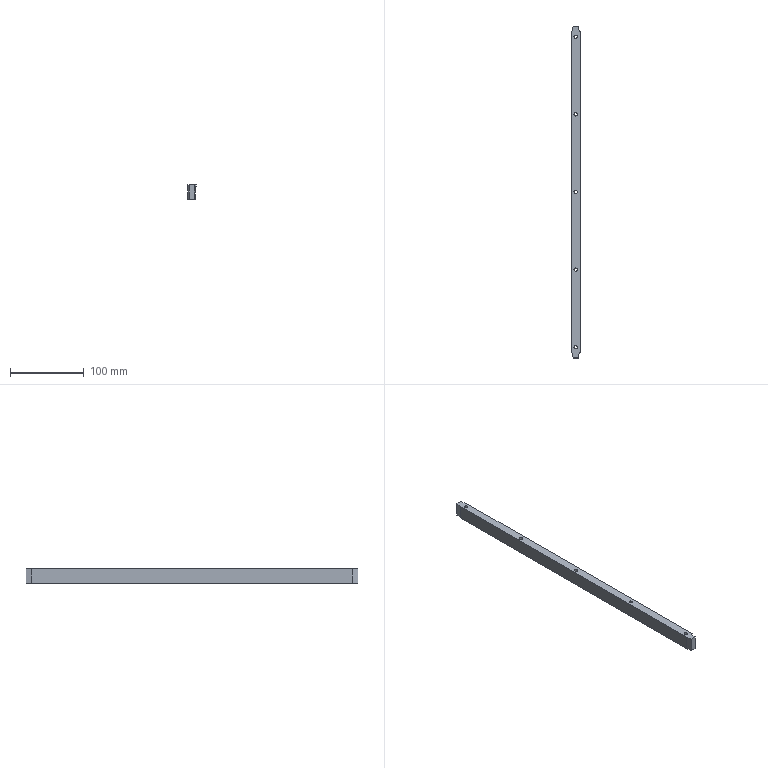Part | STEP file | 11-FG-SZ00211 | 1 solid | 39 faces | box 11 x 449 x 19 mm | volume 83756 mm3 | cylinder 20 | plane 19 | commonest cylinder face diameters 4.5 x10 8 x10
STEP:
#1=CARTESIAN_POINT('',(4.,0.,4.4));
#2=VERTEX_POINT('',#1);
#3=CARTESIAN_POINT('',(-4.,0.,4.4));
#4=VERTEX_POINT('',#3);
#5=CARTESIAN_POINT('',(0.,0.,4.4));
#6=DIRECTION('',(0.,0.,-1.));
#7=DIRECTION('',(-1.,0.,0.));
#8=AXIS2_PLACEMENT_3D('',#5,#6,#7);
#9=CIRCLE('',#8,4.);
#10=EDGE_CURVE('',#2,#4,#9,.T.);
#11=ORIENTED_EDGE('',*,*,#10,.F.);
#12=CARTESIAN_POINT('',(4.,0.,0.));
#13=VERTEX_POINT('',#12);
#14=CARTESIAN_POINT('',(4.,0.,0.));
#15=DIRECTION('',(0.,0.,-1.));
#16=VECTOR('',#15,1000.);
#17=LINE('',#14,#16);
#18=EDGE_CURVE('',#2,#13,#17,.T.);
#19=ORIENTED_EDGE('',*,*,#18,.T.);
#20=CARTESIAN_POINT('',(-4.,0.,0.));
#21=VERTEX_POINT('',#20);
#22=CARTESIAN_POINT('',(0.,0.,0.));
#23=DIRECTION('',(0.,0.,-1.));
#24=DIRECTION('',(-1.,0.,0.));
#25=AXIS2_PLACEMENT_3D('',#22,#23,#24);
#26=CIRCLE('',#25,4.);
#27=EDGE_CURVE('',#13,#21,#26,.T.);
#28=ORIENTED_EDGE('',*,*,#27,.T.);
#29=CARTESIAN_POINT('',(-4.,0.,0.));
#30=DIRECTION('',(0.,0.,-1.));
#31=VECTOR('',#30,1000.);
#32=LINE('',#29,#31);
#33=EDGE_CURVE('',#4,#21,#32,.T.);
#34=ORIENTED_EDGE('',*,*,#33,.F.);
#35=EDGE_LOOP('',(#11,#19,#28,#34));
#36=FACE_OUTER_BOUND('',#35,.T.);
#37=CARTESIAN_POINT('',(0.,0.,0.));
#38=DIRECTION('',(0.,0.,-1.));
#39=DIRECTION('',(-1.,0.,0.));
#40=AXIS2_PLACEMENT_3D('',#37,#38,#39);
#41=CYLINDRICAL_SURFACE('',#40,4.);
#42=ADVANCED_FACE('',(#36),#41,.F.);
#43=CARTESIAN_POINT('',(2.25,0.,19.));
#44=VERTEX_POINT('',#43);
#45=CARTESIAN_POINT('',(-2.25,0.,19.));
#46=VERTEX_POINT('',#45);
#47=CARTESIAN_POINT('',(0.,0.,19.));
#48=DIRECTION('',(0.,0.,-1.));
#49=DIRECTION('',(-1.,0.,0.));
#50=AXIS2_PLACEMENT_3D('',#47,#48,#49);
#51=CIRCLE('',#50,2.25);
#52=EDGE_CURVE('',#44,#46,#51,.T.);
#53=ORIENTED_EDGE('',*,*,#52,.F.);
#54=CARTESIAN_POINT('',(2.25,0.,4.4));
#55=VERTEX_POINT('',#54);
#56=CARTESIAN_POINT('',(2.25,0.,0.));
#57=DIRECTION('',(0.,0.,-1.));
#58=VECTOR('',#57,1000.);
#59=LINE('',#56,#58);
#60=EDGE_CURVE('',#44,#55,#59,.T.);
#61=ORIENTED_EDGE('',*,*,#60,.T.);
#62=CARTESIAN_POINT('',(-2.25,0.,4.4));
#63=VERTEX_POINT('',#62);
#64=CARTESIAN_POINT('',(0.,0.,4.4));
#65=DIRECTION('',(0.,0.,-1.));
#66=DIRECTION('',(-1.,0.,0.));
#67=AXIS2_PLACEMENT_3D('',#64,#65,#66);
#68=CIRCLE('',#67,2.25);
#69=EDGE_CURVE('',#55,#63,#68,.T.);
#70=ORIENTED_EDGE('',*,*,#69,.T.);
#71=CARTESIAN_POINT('',(-2.25,0.,0.));
#72=DIRECTION('',(0.,0.,-1.));
#73=VECTOR('',#72,1000.);
#74=LINE('',#71,#73);
#75=EDGE_CURVE('',#46,#63,#74,.T.);
#76=ORIENTED_EDGE('',*,*,#75,.F.);
#77=EDGE_LOOP('',(#53,#61,#70,#76));
#78=FACE_OUTER_BOUND('',#77,.T.);
#79=CARTESIAN_POINT('',(0.,0.,0.));
#80=DIRECTION('',(0.,0.,-1.));
#81=DIRECTION('',(-1.,0.,0.));
#82=AXIS2_PLACEMENT_3D('',#79,#80,#81);
#83=CYLINDRICAL_SURFACE('',#82,2.25);
#84=ADVANCED_FACE('',(#78),#83,.F.);
#85=CARTESIAN_POINT('',(4.,-105.,4.4));
#86=VERTEX_POINT('',#85);
#87=CARTESIAN_POINT('',(-4.,-105.,4.4));
#88=VERTEX_POINT('',#87);
#89=CARTESIAN_POINT('',(0.,-105.,4.4));
#90=DIRECTION('',(0.,0.,-1.));
#91=DIRECTION('',(-1.,0.,0.));
#92=AXIS2_PLACEMENT_3D('',#89,#90,#91);
#93=CIRCLE('',#92,4.);
#94=EDGE_CURVE('',#86,#88,#93,.T.);
#95=ORIENTED_EDGE('',*,*,#94,.F.);
#96=CARTESIAN_POINT('',(4.,-105.,0.));
#97=VERTEX_POINT('',#96);
#98=CARTESIAN_POINT('',(4.,-105.,0.));
#99=DIRECTION('',(0.,0.,-1.));
#100=VECTOR('',#99,1000.);
#101=LINE('',#98,#100);
#102=EDGE_CURVE('',#86,#97,#101,.T.);
#103=ORIENTED_EDGE('',*,*,#102,.T.);
#104=CARTESIAN_POINT('',(-4.,-105.,0.));
#105=VERTEX_POINT('',#104);
#106=CARTESIAN_POINT('',(0.,-105.,0.));
#107=DIRECTION('',(0.,0.,-1.));
#108=DIRECTION('',(-1.,0.,0.));
#109=AXIS2_PLACEMENT_3D('',#106,#107,#108);
#110=CIRCLE('',#109,4.);
#111=EDGE_CURVE('',#97,#105,#110,.T.);
#112=ORIENTED_EDGE('',*,*,#111,.T.);
#113=CARTESIAN_POINT('',(-4.,-105.,0.));
#114=DIRECTION('',(0.,0.,-1.));
#115=VECTOR('',#114,1000.);
#116=LINE('',#113,#115);
#117=EDGE_CURVE('',#88,#105,#116,.T.);
#118=ORIENTED_EDGE('',*,*,#117,.F.);
#119=EDGE_LOOP('',(#95,#103,#112,#118));
#120=FACE_OUTER_BOUND('',#119,.T.);
#121=CARTESIAN_POINT('',(0.,-105.,0.));
#122=DIRECTION('',(0.,0.,-1.));
#123=DIRECTION('',(-1.,0.,0.));
#124=AXIS2_PLACEMENT_3D('',#121,#122,#123);
#125=CYLINDRICAL_SURFACE('',#124,4.);
#126=ADVANCED_FACE('',(#120),#125,.F.);
#127=CARTESIAN_POINT('',(2.25,-105.,19.));
#128=VERTEX_POINT('',#127);
#129=CARTESIAN_POINT('',(-2.25,-105.,19.));
#130=VERTEX_POINT('',#129);
#131=CARTESIAN_POINT('',(0.,-105.,19.));
#132=DIRECTION('',(0.,0.,-1.));
#133=DIRECTION('',(-1.,0.,0.));
#134=AXIS2_PLACEMENT_3D('',#131,#132,#133);
#135=CIRCLE('',#134,2.25);
#136=EDGE_CURVE('',#128,#130,#135,.T.);
#137=ORIENTED_EDGE('',*,*,#136,.F.);
#138=CARTESIAN_POINT('',(2.25,-105.,4.4));
#139=VERTEX_POINT('',#138);
#140=CARTESIAN_POINT('',(2.25,-105.,0.));
#141=DIRECTION('',(0.,0.,-1.));
#142=VECTOR('',#141,1000.);
#143=LINE('',#140,#142);
#144=EDGE_CURVE('',#128,#139,#143,.T.);
#145=ORIENTED_EDGE('',*,*,#144,.T.);
#146=CARTESIAN_POINT('',(-2.25,-105.,4.4));
#147=VERTEX_POINT('',#146);
#148=CARTESIAN_POINT('',(0.,-105.,4.4));
#149=DIRECTION('',(0.,0.,-1.));
#150=DIRECTION('',(-1.,0.,0.));
#151=AXIS2_PLACEMENT_3D('',#148,#149,#150);
#152=CIRCLE('',#151,2.25);
#153=EDGE_CURVE('',#139,#147,#152,.T.);
#154=ORIENTED_EDGE('',*,*,#153,.T.);
#155=CARTESIAN_POINT('',(-2.25,-105.,0.));
#156=DIRECTION('',(0.,0.,-1.));
#157=VECTOR('',#156,1000.);
#158=LINE('',#155,#157);
#159=EDGE_CURVE('',#130,#147,#158,.T.);
#160=ORIENTED_EDGE('',*,*,#159,.F.);
#161=EDGE_LOOP('',(#137,#145,#154,#160));
#162=FACE_OUTER_BOUND('',#161,.T.);
#163=CARTESIAN_POINT('',(0.,-105.,0.));
#164=DIRECTION('',(0.,0.,-1.));
#165=DIRECTION('',(-1.,0.,0.));
#166=AXIS2_PLACEMENT_3D('',#163,#164,#165);
#167=CYLINDRICAL_SURFACE('',#166,2.25);
#168=ADVANCED_FACE('',(#162),#167,.F.);
#169=CARTESIAN_POINT('',(4.,105.,4.4));
#170=VERTEX_POINT('',#169);
#171=CARTESIAN_POINT('',(-4.,105.,4.4));
#172=VERTEX_POINT('',#171);
#173=CARTESIAN_POINT('',(0.,105.,4.4));
#174=DIRECTION('',(0.,0.,-1.));
#175=DIRECTION('',(-1.,0.,0.));
#176=AXIS2_PLACEMENT_3D('',#173,#174,#175);
#177=CIRCLE('',#176,4.);
#178=EDGE_CURVE('',#170,#172,#177,.T.);
#179=ORIENTED_EDGE('',*,*,#178,.F.);
#180=CARTESIAN_POINT('',(4.,105.,0.));
#181=VERTEX_POINT('',#180);
#182=CARTESIAN_POINT('',(4.,105.,0.));
#183=DIRECTION('',(0.,0.,-1.));
#184=VECTOR('',#183,1000.);
#185=LINE('',#182,#184);
#186=EDGE_CURVE('',#170,#181,#185,.T.);
#187=ORIENTED_EDGE('',*,*,#186,.T.);
#188=CARTESIAN_POINT('',(-4.,105.,0.));
#189=VERTEX_POINT('',#188);
#190=CARTESIAN_POINT('',(0.,105.,0.));
#191=DIRECTION('',(0.,0.,-1.));
#192=DIRECTION('',(-1.,0.,0.));
#193=AXIS2_PLACEMENT_3D('',#190,#191,#192);
#194=CIRCLE('',#193,4.);
#195=EDGE_CURVE('',#181,#189,#194,.T.);
#196=ORIENTED_EDGE('',*,*,#195,.T.);
#197=CARTESIAN_POINT('',(-4.,105.,0.));
#198=DIRECTION('',(0.,0.,-1.));
#199=VECTOR('',#198,1000.);
#200=LINE('',#197,#199);
#201=EDGE_CURVE('',#172,#189,#200,.T.);
#202=ORIENTED_EDGE('',*,*,#201,.F.);
#203=EDGE_LOOP('',(#179,#187,#196,#202));
#204=FACE_OUTER_BOUND('',#203,.T.);
#205=CARTESIAN_POINT('',(0.,105.,0.));
#206=DIRECTION('',(0.,0.,-1.));
#207=DIRECTION('',(-1.,0.,0.));
#208=AXIS2_PLACEMENT_3D('',#205,#206,#207);
#209=CYLINDRICAL_SURFACE('',#208,4.);
#210=ADVANCED_FACE('',(#204),#209,.F.);
#211=CARTESIAN_POINT('',(2.25,105.,19.));
#212=VERTEX_POINT('',#211);
#213=CARTESIAN_POINT('',(-2.25,105.,19.));
#214=VERTEX_POINT('',#213);
#215=CARTESIAN_POINT('',(0.,105.,19.));
#216=DIRECTION('',(0.,0.,-1.));
#217=DIRECTION('',(-1.,0.,0.));
#218=AXIS2_PLACEMENT_3D('',#215,#216,#217);
#219=CIRCLE('',#218,2.25);
#220=EDGE_CURVE('',#212,#214,#219,.T.);
#221=ORIENTED_EDGE('',*,*,#220,.F.);
#222=CARTESIAN_POINT('',(2.25,105.,4.4));
#223=VERTEX_POINT('',#222);
#224=CARTESIAN_POINT('',(2.25,105.,0.));
#225=DIRECTION('',(0.,0.,-1.));
#226=VECTOR('',#225,1000.);
#227=LINE('',#224,#226);
#228=EDGE_CURVE('',#212,#223,#227,.T.);
#229=ORIENTED_EDGE('',*,*,#228,.T.);
#230=CARTESIAN_POINT('',(-2.25,105.,4.4));
#231=VERTEX_POINT('',#230);
#232=CARTESIAN_POINT('',(0.,105.,4.4));
#233=DIRECTION('',(0.,0.,-1.));
#234=DIRECTION('',(-1.,0.,0.));
#235=AXIS2_PLACEMENT_3D('',#232,#233,#234);
#236=CIRCLE('',#235,2.25);
#237=EDGE_CURVE('',#223,#231,#236,.T.);
#238=ORIENTED_EDGE('',*,*,#237,.T.);
#239=CARTESIAN_POINT('',(-2.25,105.,0.));
#240=DIRECTION('',(0.,0.,-1.));
#241=VECTOR('',#240,1000.);
#242=LINE('',#239,#241);
#243=EDGE_CURVE('',#214,#231,#242,.T.);
#244=ORIENTED_EDGE('',*,*,#243,.F.);
#245=EDGE_LOOP('',(#221,#229,#238,#244));
#246=FACE_OUTER_BOUND('',#245,.T.);
#247=CARTESIAN_POINT('',(0.,105.,0.));
#248=DIRECTION('',(0.,0.,-1.));
#249=DIRECTION('',(-1.,0.,0.));
#250=AXIS2_PLACEMENT_3D('',#247,#248,#249);
#251=CYLINDRICAL_SURFACE('',#250,2.25);
#252=ADVANCED_FACE('',(#246),#251,.F.);
#253=CARTESIAN_POINT('',(4.,-210.,4.4));
#254=VERTEX_POINT('',#253);
#255=CARTESIAN_POINT('',(-4.,-210.,4.4));
#256=VERTEX_POINT('',#255);
#257=CARTESIAN_POINT('',(0.,-210.,4.4));
#258=DIRECTION('',(0.,0.,-1.));
#259=DIRECTION('',(-1.,0.,0.));
#260=AXIS2_PLACEMENT_3D('',#257,#258,#259);
#261=CIRCLE('',#260,4.);
#262=EDGE_CURVE('',#254,#256,#261,.T.);
#263=ORIENTED_EDGE('',*,*,#262,.F.);
#264=CARTESIAN_POINT('',(4.,-210.,0.));
#265=VERTEX_POINT('',#264);
#266=CARTESIAN_POINT('',(4.,-210.,0.));
#267=DIRECTION('',(0.,0.,-1.));
#268=VECTOR('',#267,1000.);
#269=LINE('',#266,#268);
#270=EDGE_CURVE('',#254,#265,#269,.T.);
#271=ORIENTED_EDGE('',*,*,#270,.T.);
#272=CARTESIAN_POINT('',(-4.,-210.,0.));
#273=VERTEX_POINT('',#272);
#274=CARTESIAN_POINT('',(0.,-210.,0.));
#275=DIRECTION('',(0.,0.,-1.));
#276=DIRECTION('',(-1.,0.,0.));
#277=AXIS2_PLACEMENT_3D('',#274,#275,#276);
#278=CIRCLE('',#277,4.);
#279=EDGE_CURVE('',#265,#273,#278,.T.);
#280=ORIENTED_EDGE('',*,*,#279,.T.);
#281=CARTESIAN_POINT('',(-4.,-210.,0.));
#282=DIRECTION('',(0.,0.,-1.));
#283=VECTOR('',#282,1000.);
#284=LINE('',#281,#283);
#285=EDGE_CURVE('',#256,#273,#284,.T.);
#286=ORIENTED_EDGE('',*,*,#285,.F.);
#287=EDGE_LOOP('',(#263,#271,#280,#286));
#288=FACE_OUTER_BOUND('',#287,.T.);
#289=CARTESIAN_POINT('',(0.,-210.,0.));
#290=DIRECTION('',(0.,0.,-1.));
#291=DIRECTION('',(-1.,0.,0.));
#292=AXIS2_PLACEMENT_3D('',#289,#290,#291);
#293=CYLINDRICAL_SURFACE('',#292,4.);
#294=ADVANCED_FACE('',(#288),#293,.F.);
#295=CARTESIAN_POINT('',(2.25,-210.,19.));
#296=VERTEX_POINT('',#295);
#297=CARTESIAN_POINT('',(-2.25,-210.,19.));
#298=VERTEX_POINT('',#297);
#299=CARTESIAN_POINT('',(0.,-210.,19.));
#300=DIRECTION('',(0.,0.,-1.));
#301=DIRECTION('',(-1.,0.,0.));
#302=AXIS2_PLACEMENT_3D('',#299,#300,#301);
#303=CIRCLE('',#302,2.25);
#304=EDGE_CURVE('',#296,#298,#303,.T.);
#305=ORIENTED_EDGE('',*,*,#304,.F.);
#306=CARTESIAN_POINT('',(2.25,-210.,4.4));
#307=VERTEX_POINT('',#306);
#308=CARTESIAN_POINT('',(2.25,-210.,0.));
#309=DIRECTION('',(0.,0.,-1.));
#310=VECTOR('',#309,1000.);
#311=LINE('',#308,#310);
#312=EDGE_CURVE('',#296,#307,#311,.T.);
#313=ORIENTED_EDGE('',*,*,#312,.T.);
#314=CARTESIAN_POINT('',(-2.25,-210.,4.4));
#315=VERTEX_POINT('',#314);
#316=CARTESIAN_POINT('',(0.,-210.,4.4));
#317=DIRECTION('',(0.,0.,-1.));
#318=DIRECTION('',(-1.,0.,0.));
#319=AXIS2_PLACEMENT_3D('',#316,#317,#318);
#320=CIRCLE('',#319,2.25);
#321=EDGE_CURVE('',#307,#315,#320,.T.);
#322=ORIENTED_EDGE('',*,*,#321,.T.);
#323=CARTESIAN_POINT('',(-2.25,-210.,0.));
#324=DIRECTION('',(0.,0.,-1.));
#325=VECTOR('',#324,1000.);
#326=LINE('',#323,#325);
#327=EDGE_CURVE('',#298,#315,#326,.T.);
#328=ORIENTED_EDGE('',*,*,#327,.F.);
#329=EDGE_LOOP('',(#305,#313,#322,#328));
#330=FACE_OUTER_BOUND('',#329,.T.);
#331=CARTESIAN_POINT('',(0.,-210.,0.));
#332=DIRECTION('',(0.,0.,-1.));
#333=DIRECTION('',(-1.,0.,0.));
#334=AXIS2_PLACEMENT_3D('',#331,#332,#333);
#335=CYLINDRICAL_SURFACE('',#334,2.25);
#336=ADVANCED_FACE('',(#330),#335,.F.);
#337=CARTESIAN_POINT('',(4.,210.,4.4));
#338=VERTEX_POINT('',#337);
#339=CARTESIAN_POINT('',(-4.,210.,4.4));
#340=VERTEX_POINT('',#339);
#341=CARTESIAN_POINT('',(0.,210.,4.4));
#342=DIRECTION('',(0.,0.,-1.));
#343=DIRECTION('',(-1.,0.,0.));
#344=AXIS2_PLACEMENT_3D('',#341,#342,#343);
#345=CIRCLE('',#344,4.);
#346=EDGE_CURVE('',#338,#340,#345,.T.);
#347=ORIENTED_EDGE('',*,*,#346,.F.);
#348=CARTESIAN_POINT('',(4.,210.,0.));
#349=VERTEX_POINT('',#348);
#350=CARTESIAN_POINT('',(4.,210.,0.));
#351=DIRECTION('',(0.,0.,-1.));
#352=VECTOR('',#351,1000.);
#353=LINE('',#350,#352);
#354=EDGE_CURVE('',#338,#349,#353,.T.);
#355=ORIENTED_EDGE('',*,*,#354,.T.);
#356=CARTESIAN_POINT('',(-4.,210.,0.));
#357=VERTEX_POINT('',#356);
#358=CARTESIAN_POINT('',(0.,210.,0.));
#359=DIRECTION('',(0.,0.,-1.));
#360=DIRECTION('',(-1.,0.,0.));
#361=AXIS2_PLACEMENT_3D('',#358,#359,#360);
#362=CIRCLE('',#361,4.);
#363=EDGE_CURVE('',#349,#357,#362,.T.);
#364=ORIENTED_EDGE('',*,*,#363,.T.);
#365=CARTESIAN_POINT('',(-4.,210.,0.));
#366=DIRECTION('',(0.,0.,-1.));
#367=VECTOR('',#366,1000.);
#368=LINE('',#365,#367);
#369=EDGE_CURVE('',#340,#357,#368,.T.);
#370=ORIENTED_EDGE('',*,*,#369,.F.);
#371=EDGE_LOOP('',(#347,#355,#364,#370));
#372=FACE_OUTER_BOUND('',#371,.T.);
#373=CARTESIAN_POINT('',(0.,210.,0.));
#374=DIRECTION('',(0.,0.,-1.));
#375=DIRECTION('',(-1.,0.,0.));
#376=AXIS2_PLACEMENT_3D('',#373,#374,#375);
#377=CYLINDRICAL_SURFACE('',#376,4.);
#378=ADVANCED_FACE('',(#372),#377,.F.);
#379=CARTESIAN_POINT('',(2.25,210.,19.));
#380=VERTEX_POINT('',#379);
#381=CARTESIAN_POINT('',(-2.25,210.,19.));
#382=VERTEX_POINT('',#381);
#383=CARTESIAN_POINT('',(0.,210.,19.));
#384=DIRECTION('',(0.,0.,-1.));
#385=DIRECTION('',(-1.,0.,0.));
#386=AXIS2_PLACEMENT_3D('',#383,#384,#385);
#387=CIRCLE('',#386,2.25);
#388=EDGE_CURVE('',#380,#382,#387,.T.);
#389=ORIENTED_EDGE('',*,*,#388,.F.);
#390=CARTESIAN_POINT('',(2.25,210.,4.4));
#391=VERTEX_POINT('',#390);
#392=CARTESIAN_POINT('',(2.25,210.,0.));
#393=DIRECTION('',(0.,0.,-1.));
#394=VECTOR('',#393,1000.);
#395=LINE('',#392,#394);
#396=EDGE_CURVE('',#380,#391,#395,.T.);
#397=ORIENTED_EDGE('',*,*,#396,.T.);
#398=CARTESIAN_POINT('',(-2.25,210.,4.4));
#399=VERTEX_POINT('',#398);
#400=CARTESIAN_POINT('',(0.,210.,4.4));
#401=DIRECTION('',(0.,0.,-1.));
#402=DIRECTION('',(-1.,0.,0.));
#403=AXIS2_PLACEMENT_3D('',#400,#401,#402);
#404=CIRCLE('',#403,2.25);
#405=EDGE_CURVE('',#391,#399,#404,.T.);
#406=ORIENTED_EDGE('',*,*,#405,.T.);
#407=CARTESIAN_POINT('',(-2.25,210.,0.));
#408=DIRECTION('',(0.,0.,-1.));
#409=VECTOR('',#408,1000.);
#410=LINE('',#407,#409);
#411=EDGE_CURVE('',#382,#399,#410,.T.);
#412=ORIENTED_EDGE('',*,*,#411,.F.);
#413=EDGE_LOOP('',(#389,#397,#406,#412));
#414=FACE_OUTER_BOUND('',#413,.T.);
#415=CARTESIAN_POINT('',(0.,210.,0.));
#416=DIRECTION('',(0.,0.,-1.));
#417=DIRECTION('',(-1.,0.,0.));
#418=AXIS2_PLACEMENT_3D('',#415,#416,#417);
#419=CYLINDRICAL_SURFACE('',#418,2.25);
#420=ADVANCED_FACE('',(#414),#419,.F.);
#421=CARTESIAN_POINT('',(5.,-216.5,16.3));
#422=VERTEX_POINT('',#421);
#423=CARTESIAN_POINT('',(5.,216.5,16.3));
#424=VERTEX_POINT('',#423);
#425=CARTESIAN_POINT('',(5.,-216.5,16.3));
#426=DIRECTION('',(0.,1.,0.));
#427=VECTOR('',#426,1000.);
#428=LINE('',#425,#427);
#429=EDGE_CURVE('',#422,#424,#428,.T.);
#430=ORIENTED_EDGE('',*,*,#429,.F.);
#431=CARTESIAN_POINT('',(5.,-216.5,0.));
#432=VERTEX_POINT('',#431);
#433=CARTESIAN_POINT('',(5.,-216.5,19.));
#434=DIRECTION('',(0.,0.,-1.));
#435=VECTOR('',#434,1000.);
#436=LINE('',#433,#435);
#437=EDGE_CURVE('',#422,#432,#436,.T.);
#438=ORIENTED_EDGE('',*,*,#437,.T.);
#439=CARTESIAN_POINT('',(5.,216.5,0.));
#440=VERTEX_POINT('',#439);
#441=CARTESIAN_POINT('',(5.,224.5,0.));
#442=DIRECTION('',(0.,1.,0.));
#443=VECTOR('',#442,1000.);
#444=LINE('',#441,#443);
#445=EDGE_CURVE('',#432,#440,#444,.T.);
#446=ORIENTED_EDGE('',*,*,#445,.T.);
#447=CARTESIAN_POINT('',(5.,216.5,19.));
#448=DIRECTION('',(0.,0.,1.));
#449=VECTOR('',#448,1000.);
#450=LINE('',#447,#449);
#451=EDGE_CURVE('',#440,#424,#450,.T.);
#452=ORIENTED_EDGE('',*,*,#451,.T.);
#453=EDGE_LOOP('',(#430,#438,#446,#452));
#454=FACE_OUTER_BOUND('',#453,.T.);
#455=CARTESIAN_POINT('',(5.,224.5,19.));
#456=DIRECTION('',(-1.,0.,0.));
#457=DIRECTION('',(0.,-1.,0.));
#458=AXIS2_PLACEMENT_3D('',#455,#456,#457);
#459=PLANE('',#458);
#460=ADVANCED_FACE('',(#454),#459,.F.);
#461=CARTESIAN_POINT('',(-5.,216.5,0.));
#462=VERTEX_POINT('',#461);
#463=CARTESIAN_POINT('',(-5.,-216.5,0.));
#464=VERTEX_POINT('',#463);
#465=CARTESIAN_POINT('',(-5.,224.5,0.));
#466=DIRECTION('',(0.,-1.,0.));
#467=VECTOR('',#466,1000.);
#468=LINE('',#465,#467);
#469=EDGE_CURVE('',#462,#464,#468,.T.);
#470=ORIENTED_EDGE('',*,*,#469,.T.);
#471=CARTESIAN_POINT('',(-5.,-216.5,19.));
#472=VERTEX_POINT('',#471);
#473=CARTESIAN_POINT('',(-5.,-216.5,19.));
#474=DIRECTION('',(0.,0.,1.));
#475=VECTOR('',#474,1000.);
#476=LINE('',#473,#475);
#477=EDGE_CURVE('',#464,#472,#476,.T.);
#478=ORIENTED_EDGE('',*,*,#477,.T.);
#479=CARTESIAN_POINT('',(-5.,216.5,19.));
#480=VERTEX_POINT('',#479);
#481=CARTESIAN_POINT('',(-5.,224.5,19.));
#482=DIRECTION('',(0.,-1.,0.));
#483=VECTOR('',#482,1000.);
#484=LINE('',#481,#483);
#485=EDGE_CURVE('',#480,#472,#484,.T.);
#486=ORIENTED_EDGE('',*,*,#485,.F.);
#487=CARTESIAN_POINT('',(-5.,216.5,19.));
#488=DIRECTION('',(0.,0.,-1.));
#489=VECTOR('',#488,1000.);
#490=LINE('',#487,#489);
#491=EDGE_CURVE('',#480,#462,#490,.T.);
#492=ORIENTED_EDGE('',*,*,#491,.T.);
#493=EDGE_LOOP('',(#470,#478,#486,#492));
#494=FACE_OUTER_BOUND('',#493,.T.);
#495=CARTESIAN_POINT('',(-5.,224.5,19.));
#496=DIRECTION('',(1.,0.,0.));
#497=DIRECTION('',(0.,1.,0.));
#498=AXIS2_PLACEMENT_3D('',#495,#496,#497);
#499=PLANE('',#498);
#500=ADVANCED_FACE('',(#494),#499,.F.);
#501=CARTESIAN_POINT('',(-3.5,-224.5,19.));
#502=VERTEX_POINT('',#501);
#503=CARTESIAN_POINT('',(3.5,-224.5,19.));
#504=VERTEX_POINT('',#503);
#505=CARTESIAN_POINT('',(5.,-224.5,19.));
#506=DIRECTION('',(1.,0.,0.));
#507=VECTOR('',#506,1000.);
#508=LINE('',#505,#507);
#509=EDGE_CURVE('',#502,#504,#508,.T.);
#510=ORIENTED_EDGE('',*,*,#509,.F.);
#511=CARTESIAN_POINT('',(-3.5,-224.5,0.));
#512=VERTEX_POINT('',#511);
#513=CARTESIAN_POINT('',(-3.5,-224.5,19.));
#514=DIRECTION('',(0.,0.,-1.));
#515=VECTOR('',#514,1000.);
#516=LINE('',#513,#515);
#517=EDGE_CURVE('',#502,#512,#516,.T.);
#518=ORIENTED_EDGE('',*,*,#517,.T.);
#519=CARTESIAN_POINT('',(3.5,-224.5,0.));
#520=VERTEX_POINT('',#519);
#521=CARTESIAN_POINT('',(5.,-224.5,0.));
#522=DIRECTION('',(1.,0.,0.));
#523=VECTOR('',#522,1000.);
#524=LINE('',#521,#523);
#525=EDGE_CURVE('',#512,#520,#524,.T.);
#526=ORIENTED_EDGE('',*,*,#525,.T.);
#527=CARTESIAN_POINT('',(3.5,-224.5,19.));
#528=DIRECTION('',(0.,0.,1.));
#529=VECTOR('',#528,1000.);
#530=LINE('',#527,#529);
#531=EDGE_CURVE('',#520,#504,#530,.T.);
#532=ORIENTED_EDGE('',*,*,#531,.T.);
#533=EDGE_LOOP('',(#510,#518,#526,#532));
#534=FACE_OUTER_BOUND('',#533,.T.);
#535=CARTESIAN_POINT('',(5.,-224.5,19.));
#536=DIRECTION('',(0.,1.,0.));
#537=DIRECTION('',(0.,0.,1.));
#538=AXIS2_PLACEMENT_3D('',#535,#536,#537);
#539=PLANE('',#538);
#540=ADVANCED_FACE('',(#534),#539,.F.);
#541=CARTESIAN_POINT('',(3.5,224.5,19.));
#542=VERTEX_POINT('',#541);
#543=CARTESIAN_POINT('',(-3.5,224.5,19.));
#544=VERTEX_POINT('',#543);
#545=CARTESIAN_POINT('',(5.,224.5,19.));
#546=DIRECTION('',(-1.,0.,0.));
#547=VECTOR('',#546,1000.);
#548=LINE('',#545,#547);
#549=EDGE_CURVE('',#542,#544,#548,.T.);
#550=ORIENTED_EDGE('',*,*,#549,.F.);
#551=CARTESIAN_POINT('',(3.5,224.5,0.));
#552=VERTEX_POINT('',#551);
#553=CARTESIAN_POINT('',(3.5,224.5,19.));
#554=DIRECTION('',(0.,0.,-1.));
#555=VECTOR('',#554,1000.);
#556=LINE('',#553,#555);
#557=EDGE_CURVE('',#542,#552,#556,.T.);
#558=ORIENTED_EDGE('',*,*,#557,.T.);
#559=CARTESIAN_POINT('',(-3.5,224.5,0.));
#560=VERTEX_POINT('',#559);
#561=CARTESIAN_POINT('',(5.,224.5,0.));
#562=DIRECTION('',(-1.,0.,0.));
#563=VECTOR('',#562,1000.);
#564=LINE('',#561,#563);
#565=EDGE_CURVE('',#552,#560,#564,.T.);
#566=ORIENTED_EDGE('',*,*,#565,.T.);
#567=CARTESIAN_POINT('',(-3.5,224.5,19.));
#568=DIRECTION('',(0.,0.,1.));
#569=VECTOR('',#568,1000.);
#570=LINE('',#567,#569);
#571=EDGE_CURVE('',#560,#544,#570,.T.);
#572=ORIENTED_EDGE('',*,*,#571,.T.);
#573=EDGE_LOOP('',(#550,#558,#566,#572));
#574=FACE_OUTER_BOUND('',#573,.T.);
#575=CARTESIAN_POINT('',(5.,224.5,19.));
#576=DIRECTION('',(0.,-1.,0.));
#577=DIRECTION('',(0.,0.,-1.));
#578=AXIS2_PLACEMENT_3D('',#575,#576,#577);
#579=PLANE('',#578);
#580=ADVANCED_FACE('',(#574),#579,.F.);
#581=CARTESIAN_POINT('',(0.,0.,19.));
#582=DIRECTION('',(0.,0.,-1.));
#583=DIRECTION('',(-1.,0.,0.));
#584=AXIS2_PLACEMENT_3D('',#581,#582,#583);
#585=CIRCLE('',#584,2.25);
#586=EDGE_CURVE('',#46,#44,#585,.T.);
#587=ORIENTED_EDGE('',*,*,#586,.T.);
#588=ORIENTED_EDGE('',*,*,#52,.T.);
#589=EDGE_LOOP('',(#587,#588));
#590=FACE_BOUND('',#589,.T.);
#591=CARTESIAN_POINT('',(0.,-105.,19.));
#592=DIRECTION('',(0.,0.,-1.));
#593=DIRECTION('',(-1.,0.,0.));
#594=AXIS2_PLACEMENT_3D('',#591,#592,#593);
#595=CIRCLE('',#594,2.25);
#596=EDGE_CURVE('',#130,#128,#595,.T.);
#597=ORIENTED_EDGE('',*,*,#596,.T.);
#598=ORIENTED_EDGE('',*,*,#136,.T.);
#599=EDGE_LOOP('',(#597,#598));
#600=FACE_BOUND('',#599,.T.);
#601=CARTESIAN_POINT('',(0.,105.,19.));
#602=DIRECTION('',(0.,0.,-1.));
#603=DIRECTION('',(-1.,0.,0.));
#604=AXIS2_PLACEMENT_3D('',#601,#602,#603);
#605=CIRCLE('',#604,2.25);
#606=EDGE_CURVE('',#214,#212,#605,.T.);
#607=ORIENTED_EDGE('',*,*,#606,.T.);
#608=ORIENTED_EDGE('',*,*,#220,.T.);
#609=EDGE_LOOP('',(#607,#608));
#610=FACE_BOUND('',#609,.T.);
#611=CARTESIAN_POINT('',(0.,-210.,19.));
#612=DIRECTION('',(0.,0.,-1.));
#613=DIRECTION('',(-1.,0.,0.));
#614=AXIS2_PLACEMENT_3D('',#611,#612,#613);
#615=CIRCLE('',#614,2.25);
#616=EDGE_CURVE('',#298,#296,#615,.T.);
#617=ORIENTED_EDGE('',*,*,#616,.T.);
#618=ORIENTED_EDGE('',*,*,#304,.T.);
#619=EDGE_LOOP('',(#617,#618));
#620=FACE_BOUND('',#619,.T.);
#621=CARTESIAN_POINT('',(0.,210.,19.));
#622=DIRECTION('',(0.,0.,-1.));
#623=DIRECTION('',(-1.,0.,0.));
#624=AXIS2_PLACEMENT_3D('',#621,#622,#623);
#625=CIRCLE('',#624,2.25);
#626=EDGE_CURVE('',#382,#380,#625,.T.);
#627=ORIENTED_EDGE('',*,*,#626,.T.);
#628=ORIENTED_EDGE('',*,*,#388,.T.);
#629=EDGE_LOOP('',(#627,#628));
#630=FACE_BOUND('',#629,.T.);
#631=CARTESIAN_POINT('',(5.,-216.5,19.));
#632=VERTEX_POINT('',#631);
#633=CARTESIAN_POINT('',(5.,-216.5,19.));
#634=DIRECTION('',(0.1843,0.9829,0.));
#635=VECTOR('',#634,1000.);
#636=LINE('',#633,#635);
#637=EDGE_CURVE('',#504,#632,#636,.T.);
#638=ORIENTED_EDGE('',*,*,#637,.T.);
#639=CARTESIAN_POINT('',(6.,-216.5,19.));
#640=VERTEX_POINT('',#639);
#641=CARTESIAN_POINT('',(6.,-216.5,19.));
#642=DIRECTION('',(-1.,0.,0.));
#643=VECTOR('',#642,1000.);
#644=LINE('',#641,#643);
#645=EDGE_CURVE('',#640,#632,#644,.T.);
#646=ORIENTED_EDGE('',*,*,#645,.F.);
#647=CARTESIAN_POINT('',(6.,216.5,19.));
#648=VERTEX_POINT('',#647);
#649=CARTESIAN_POINT('',(6.,-216.5,19.));
#650=DIRECTION('',(0.,-1.,0.));
#651=VECTOR('',#650,1000.);
#652=LINE('',#649,#651);
#653=EDGE_CURVE('',#648,#640,#652,.T.);
#654=ORIENTED_EDGE('',*,*,#653,.F.);
#655=CARTESIAN_POINT('',(5.,216.5,19.));
#656=VERTEX_POINT('',#655);
#657=CARTESIAN_POINT('',(6.,216.5,19.));
#658=DIRECTION('',(-1.,0.,0.));
#659=VECTOR('',#658,1000.);
#660=LINE('',#657,#659);
#661=EDGE_CURVE('',#648,#656,#660,.T.);
#662=ORIENTED_EDGE('',*,*,#661,.T.);
#663=CARTESIAN_POINT('',(3.5,224.5,19.));
#664=DIRECTION('',(-0.1843,0.9829,0.));
#665=VECTOR('',#664,1000.);
#666=LINE('',#663,#665);
#667=EDGE_CURVE('',#656,#542,#666,.T.);
#668=ORIENTED_EDGE('',*,*,#667,.T.);
#669=ORIENTED_EDGE('',*,*,#549,.T.);
#670=CARTESIAN_POINT('',(-5.,216.5,19.));
#671=DIRECTION('',(-0.1843,-0.9829,0.));
#672=VECTOR('',#671,1000.);
#673=LINE('',#670,#672);
#674=EDGE_CURVE('',#544,#480,#673,.T.);
#675=ORIENTED_EDGE('',*,*,#674,.T.);
#676=ORIENTED_EDGE('',*,*,#485,.T.);
#677=CARTESIAN_POINT('',(-3.5,-224.5,19.));
#678=DIRECTION('',(0.1843,-0.9829,0.));
#679=VECTOR('',#678,1000.);
#680=LINE('',#677,#679);
#681=EDGE_CURVE('',#472,#502,#680,.T.);
#682=ORIENTED_EDGE('',*,*,#681,.T.);
#683=ORIENTED_EDGE('',*,*,#509,.T.);
#684=EDGE_LOOP('',(#638,#646,#654,#662,#668,#669,#675,#676,#682,#683));
#685=FACE_OUTER_BOUND('',#684,.T.);
#686=CARTESIAN_POINT('',(0.,0.,19.));
#687=DIRECTION('',(0.,0.,-1.));
#688=DIRECTION('',(-1.,0.,0.));
#689=AXIS2_PLACEMENT_3D('',#686,#687,#688);
#690=PLANE('',#689);
#691=ADVANCED_FACE('',(#590,#600,#610,#620,#630,#685),#690,.F.);
#692=CARTESIAN_POINT('',(0.,0.,0.));
#693=DIRECTION('',(0.,0.,-1.));
#694=DIRECTION('',(-1.,0.,0.));
#695=AXIS2_PLACEMENT_3D('',#692,#693,#694);
#696=CIRCLE('',#695,4.);
#697=EDGE_CURVE('',#21,#13,#696,.T.);
#698=ORIENTED_EDGE('',*,*,#697,.F.);
#699=ORIENTED_EDGE('',*,*,#27,.F.);
#700=EDGE_LOOP('',(#698,#699));
#701=FACE_BOUND('',#700,.T.);
#702=CARTESIAN_POINT('',(0.,-105.,0.));
#703=DIRECTION('',(0.,0.,-1.));
#704=DIRECTION('',(-1.,0.,0.));
#705=AXIS2_PLACEMENT_3D('',#702,#703,#704);
#706=CIRCLE('',#705,4.);
#707=EDGE_CURVE('',#105,#97,#706,.T.);
#708=ORIENTED_EDGE('',*,*,#707,.F.);
#709=ORIENTED_EDGE('',*,*,#111,.F.);
#710=EDGE_LOOP('',(#708,#709));
#711=FACE_BOUND('',#710,.T.);
#712=CARTESIAN_POINT('',(0.,105.,0.));
#713=DIRECTION('',(0.,0.,-1.));
#714=DIRECTION('',(-1.,0.,0.));
#715=AXIS2_PLACEMENT_3D('',#712,#713,#714);
#716=CIRCLE('',#715,4.);
#717=EDGE_CURVE('',#189,#181,#716,.T.);
#718=ORIENTED_EDGE('',*,*,#717,.F.);
#719=ORIENTED_EDGE('',*,*,#195,.F.);
#720=EDGE_LOOP('',(#718,#719));
#721=FACE_BOUND('',#720,.T.);
#722=CARTESIAN_POINT('',(0.,-210.,0.));
#723=DIRECTION('',(0.,0.,-1.));
#724=DIRECTION('',(-1.,0.,0.));
#725=AXIS2_PLACEMENT_3D('',#722,#723,#724);
#726=CIRCLE('',#725,4.);
#727=EDGE_CURVE('',#273,#265,#726,.T.);
#728=ORIENTED_EDGE('',*,*,#727,.F.);
#729=ORIENTED_EDGE('',*,*,#279,.F.);
#730=EDGE_LOOP('',(#728,#729));
#731=FACE_BOUND('',#730,.T.);
#732=CARTESIAN_POINT('',(0.,210.,0.));
#733=DIRECTION('',(0.,0.,-1.));
#734=DIRECTION('',(-1.,0.,0.));
#735=AXIS2_PLACEMENT_3D('',#732,#733,#734);
#736=CIRCLE('',#735,4.);
#737=EDGE_CURVE('',#357,#349,#736,.T.);
#738=ORIENTED_EDGE('',*,*,#737,.F.);
#739=ORIENTED_EDGE('',*,*,#363,.F.);
#740=EDGE_LOOP('',(#738,#739));
#741=FACE_BOUND('',#740,.T.);
#742=ORIENTED_EDGE('',*,*,#565,.F.);
#743=CARTESIAN_POINT('',(44.045,8.258,0.));
#744=DIRECTION('',(0.1843,-0.9829,0.));
#745=VECTOR('',#744,1000.);
#746=LINE('',#743,#745);
#747=EDGE_CURVE('',#552,#440,#746,.T.);
#748=ORIENTED_EDGE('',*,*,#747,.T.);
#749=ORIENTED_EDGE('',*,*,#445,.F.);
#750=CARTESIAN_POINT('',(44.045,-8.258,0.));
#751=DIRECTION('',(-0.1843,-0.9829,0.));
#752=VECTOR('',#751,1000.);
#753=LINE('',#750,#752);
#754=EDGE_CURVE('',#432,#520,#753,.T.);
#755=ORIENTED_EDGE('',*,*,#754,.T.);
#756=ORIENTED_EDGE('',*,*,#525,.F.);
#757=CARTESIAN_POINT('',(-44.045,-8.258,0.));
#758=DIRECTION('',(-0.1843,0.9829,0.));
#759=VECTOR('',#758,1000.);
#760=LINE('',#757,#759);
#761=EDGE_CURVE('',#512,#464,#760,.T.);
#762=ORIENTED_EDGE('',*,*,#761,.T.);
#763=ORIENTED_EDGE('',*,*,#469,.F.);
#764=CARTESIAN_POINT('',(-44.045,8.258,0.));
#765=DIRECTION('',(0.1843,0.9829,0.));
#766=VECTOR('',#765,1000.);
#767=LINE('',#764,#766);
#768=EDGE_CURVE('',#462,#560,#767,.T.);
#769=ORIENTED_EDGE('',*,*,#768,.T.);
#770=EDGE_LOOP('',(#742,#748,#749,#755,#756,#762,#763,#769));
#771=FACE_OUTER_BOUND('',#770,.T.);
#772=CARTESIAN_POINT('',(0.,0.,0.));
#773=DIRECTION('',(0.,0.,-1.));
#774=DIRECTION('',(-1.,0.,0.));
#775=AXIS2_PLACEMENT_3D('',#772,#773,#774);
#776=PLANE('',#775);
#777=ADVANCED_FACE('',(#701,#711,#721,#731,#741,#771),#776,.T.);
#778=ORIENTED_EDGE('',*,*,#396,.F.);
#779=ORIENTED_EDGE('',*,*,#626,.F.);
#780=ORIENTED_EDGE('',*,*,#411,.T.);
#781=CARTESIAN_POINT('',(0.,210.,4.4));
#782=DIRECTION('',(0.,0.,-1.));
#783=DIRECTION('',(-1.,0.,0.));
#784=AXIS2_PLACEMENT_3D('',#781,#782,#783);
#785=CIRCLE('',#784,2.25);
#786=EDGE_CURVE('',#399,#391,#785,.T.);
#787=ORIENTED_EDGE('',*,*,#786,.T.);
#788=EDGE_LOOP('',(#778,#779,#780,#787));
#789=FACE_OUTER_BOUND('',#788,.T.);
#790=CARTESIAN_POINT('',(0.,210.,0.));
#791=DIRECTION('',(0.,0.,-1.));
#792=DIRECTION('',(-1.,0.,0.));
#793=AXIS2_PLACEMENT_3D('',#790,#791,#792);
#794=CYLINDRICAL_SURFACE('',#793,2.25);
#795=ADVANCED_FACE('',(#789),#794,.F.);
#796=ORIENTED_EDGE('',*,*,#786,.F.);
#797=ORIENTED_EDGE('',*,*,#405,.F.);
#798=EDGE_LOOP('',(#796,#797));
#799=FACE_BOUND('',#798,.T.);
#800=CARTESIAN_POINT('',(0.,210.,4.4));
#801=DIRECTION('',(0.,0.,-1.));
#802=DIRECTION('',(-1.,0.,0.));
#803=AXIS2_PLACEMENT_3D('',#800,#801,#802);
#804=CIRCLE('',#803,4.);
#805=EDGE_CURVE('',#340,#338,#804,.T.);
#806=ORIENTED_EDGE('',*,*,#805,.T.);
#807=ORIENTED_EDGE('',*,*,#346,.T.);
#808=EDGE_LOOP('',(#806,#807));
#809=FACE_OUTER_BOUND('',#808,.T.);
#810=CARTESIAN_POINT('',(2.25,210.,4.4));
#811=DIRECTION('',(0.,0.,1.));
#812=DIRECTION('',(1.,0.,0.));
#813=AXIS2_PLACEMENT_3D('',#810,#811,#812);
#814=PLANE('',#813);
#815=ADVANCED_FACE('',(#799,#809),#814,.F.);
#816=ORIENTED_EDGE('',*,*,#354,.F.);
#817=ORIENTED_EDGE('',*,*,#805,.F.);
#818=ORIENTED_EDGE('',*,*,#369,.T.);
#819=ORIENTED_EDGE('',*,*,#737,.T.);
#820=EDGE_LOOP('',(#816,#817,#818,#819));
#821=FACE_OUTER_BOUND('',#820,.T.);
#822=CARTESIAN_POINT('',(0.,210.,0.));
#823=DIRECTION('',(0.,0.,-1.));
#824=DIRECTION('',(-1.,0.,0.));
#825=AXIS2_PLACEMENT_3D('',#822,#823,#824);
#826=CYLINDRICAL_SURFACE('',#825,4.);
#827=ADVANCED_FACE('',(#821),#826,.F.);
#828=ORIENTED_EDGE('',*,*,#312,.F.);
#829=ORIENTED_EDGE('',*,*,#616,.F.);
#830=ORIENTED_EDGE('',*,*,#327,.T.);
#831=CARTESIAN_POINT('',(0.,-210.,4.4));
#832=DIRECTION('',(0.,0.,-1.));
#833=DIRECTION('',(-1.,0.,0.));
#834=AXIS2_PLACEMENT_3D('',#831,#832,#833);
#835=CIRCLE('',#834,2.25);
#836=EDGE_CURVE('',#315,#307,#835,.T.);
#837=ORIENTED_EDGE('',*,*,#836,.T.);
#838=EDGE_LOOP('',(#828,#829,#830,#837));
#839=FACE_OUTER_BOUND('',#838,.T.);
#840=CARTESIAN_POINT('',(0.,-210.,0.));
#841=DIRECTION('',(0.,0.,-1.));
#842=DIRECTION('',(-1.,0.,0.));
#843=AXIS2_PLACEMENT_3D('',#840,#841,#842);
#844=CYLINDRICAL_SURFACE('',#843,2.25);
#845=ADVANCED_FACE('',(#839),#844,.F.);
#846=ORIENTED_EDGE('',*,*,#836,.F.);
#847=ORIENTED_EDGE('',*,*,#321,.F.);
#848=EDGE_LOOP('',(#846,#847));
#849=FACE_BOUND('',#848,.T.);
#850=CARTESIAN_POINT('',(0.,-210.,4.4));
#851=DIRECTION('',(0.,0.,-1.));
#852=DIRECTION('',(-1.,0.,0.));
#853=AXIS2_PLACEMENT_3D('',#850,#851,#852);
#854=CIRCLE('',#853,4.);
#855=EDGE_CURVE('',#256,#254,#854,.T.);
#856=ORIENTED_EDGE('',*,*,#855,.T.);
#857=ORIENTED_EDGE('',*,*,#262,.T.);
#858=EDGE_LOOP('',(#856,#857));
#859=FACE_OUTER_BOUND('',#858,.T.);
#860=CARTESIAN_POINT('',(2.25,-210.,4.4));
#861=DIRECTION('',(0.,0.,1.));
#862=DIRECTION('',(1.,0.,0.));
#863=AXIS2_PLACEMENT_3D('',#860,#861,#862);
#864=PLANE('',#863);
#865=ADVANCED_FACE('',(#849,#859),#864,.F.);
#866=ORIENTED_EDGE('',*,*,#270,.F.);
#867=ORIENTED_EDGE('',*,*,#855,.F.);
#868=ORIENTED_EDGE('',*,*,#285,.T.);
#869=ORIENTED_EDGE('',*,*,#727,.T.);
#870=EDGE_LOOP('',(#866,#867,#868,#869));
#871=FACE_OUTER_BOUND('',#870,.T.);
#872=CARTESIAN_POINT('',(0.,-210.,0.));
#873=DIRECTION('',(0.,0.,-1.));
#874=DIRECTION('',(-1.,0.,0.));
#875=AXIS2_PLACEMENT_3D('',#872,#873,#874);
#876=CYLINDRICAL_SURFACE('',#875,4.);
#877=ADVANCED_FACE('',(#871),#876,.F.);
#878=ORIENTED_EDGE('',*,*,#228,.F.);
#879=ORIENTED_EDGE('',*,*,#606,.F.);
#880=ORIENTED_EDGE('',*,*,#243,.T.);
#881=CARTESIAN_POINT('',(0.,105.,4.4));
#882=DIRECTION('',(0.,0.,-1.));
#883=DIRECTION('',(-1.,0.,0.));
#884=AXIS2_PLACEMENT_3D('',#881,#882,#883);
#885=CIRCLE('',#884,2.25);
#886=EDGE_CURVE('',#231,#223,#885,.T.);
#887=ORIENTED_EDGE('',*,*,#886,.T.);
#888=EDGE_LOOP('',(#878,#879,#880,#887));
#889=FACE_OUTER_BOUND('',#888,.T.);
#890=CARTESIAN_POINT('',(0.,105.,0.));
#891=DIRECTION('',(0.,0.,-1.));
#892=DIRECTION('',(-1.,0.,0.));
#893=AXIS2_PLACEMENT_3D('',#890,#891,#892);
#894=CYLINDRICAL_SURFACE('',#893,2.25);
#895=ADVANCED_FACE('',(#889),#894,.F.);
#896=ORIENTED_EDGE('',*,*,#886,.F.);
#897=ORIENTED_EDGE('',*,*,#237,.F.);
#898=EDGE_LOOP('',(#896,#897));
#899=FACE_BOUND('',#898,.T.);
#900=CARTESIAN_POINT('',(0.,105.,4.4));
#901=DIRECTION('',(0.,0.,-1.));
#902=DIRECTION('',(-1.,0.,0.));
#903=AXIS2_PLACEMENT_3D('',#900,#901,#902);
#904=CIRCLE('',#903,4.);
#905=EDGE_CURVE('',#172,#170,#904,.T.);
#906=ORIENTED_EDGE('',*,*,#905,.T.);
#907=ORIENTED_EDGE('',*,*,#178,.T.);
#908=EDGE_LOOP('',(#906,#907));
#909=FACE_OUTER_BOUND('',#908,.T.);
#910=CARTESIAN_POINT('',(2.25,105.,4.4));
#911=DIRECTION('',(0.,0.,1.));
#912=DIRECTION('',(1.,0.,0.));
#913=AXIS2_PLACEMENT_3D('',#910,#911,#912);
#914=PLANE('',#913);
#915=ADVANCED_FACE('',(#899,#909),#914,.F.);
#916=ORIENTED_EDGE('',*,*,#186,.F.);
#917=ORIENTED_EDGE('',*,*,#905,.F.);
#918=ORIENTED_EDGE('',*,*,#201,.T.);
#919=ORIENTED_EDGE('',*,*,#717,.T.);
#920=EDGE_LOOP('',(#916,#917,#918,#919));
#921=FACE_OUTER_BOUND('',#920,.T.);
#922=CARTESIAN_POINT('',(0.,105.,0.));
#923=DIRECTION('',(0.,0.,-1.));
#924=DIRECTION('',(-1.,0.,0.));
#925=AXIS2_PLACEMENT_3D('',#922,#923,#924);
#926=CYLINDRICAL_SURFACE('',#925,4.);
#927=ADVANCED_FACE('',(#921),#926,.F.);
#928=ORIENTED_EDGE('',*,*,#144,.F.);
#929=ORIENTED_EDGE('',*,*,#596,.F.);
#930=ORIENTED_EDGE('',*,*,#159,.T.);
#931=CARTESIAN_POINT('',(0.,-105.,4.4));
#932=DIRECTION('',(0.,0.,-1.));
#933=DIRECTION('',(-1.,0.,0.));
#934=AXIS2_PLACEMENT_3D('',#931,#932,#933);
#935=CIRCLE('',#934,2.25);
#936=EDGE_CURVE('',#147,#139,#935,.T.);
#937=ORIENTED_EDGE('',*,*,#936,.T.);
#938=EDGE_LOOP('',(#928,#929,#930,#937));
#939=FACE_OUTER_BOUND('',#938,.T.);
#940=CARTESIAN_POINT('',(0.,-105.,0.));
#941=DIRECTION('',(0.,0.,-1.));
#942=DIRECTION('',(-1.,0.,0.));
#943=AXIS2_PLACEMENT_3D('',#940,#941,#942);
#944=CYLINDRICAL_SURFACE('',#943,2.25);
#945=ADVANCED_FACE('',(#939),#944,.F.);
#946=ORIENTED_EDGE('',*,*,#936,.F.);
#947=ORIENTED_EDGE('',*,*,#153,.F.);
#948=EDGE_LOOP('',(#946,#947));
#949=FACE_BOUND('',#948,.T.);
#950=CARTESIAN_POINT('',(0.,-105.,4.4));
#951=DIRECTION('',(0.,0.,-1.));
#952=DIRECTION('',(-1.,0.,0.));
#953=AXIS2_PLACEMENT_3D('',#950,#951,#952);
#954=CIRCLE('',#953,4.);
#955=EDGE_CURVE('',#88,#86,#954,.T.);
#956=ORIENTED_EDGE('',*,*,#955,.T.);
#957=ORIENTED_EDGE('',*,*,#94,.T.);
#958=EDGE_LOOP('',(#956,#957));
#959=FACE_OUTER_BOUND('',#958,.T.);
#960=CARTESIAN_POINT('',(2.25,-105.,4.4));
#961=DIRECTION('',(0.,0.,1.));
#962=DIRECTION('',(1.,0.,0.));
#963=AXIS2_PLACEMENT_3D('',#960,#961,#962);
#964=PLANE('',#963);
#965=ADVANCED_FACE('',(#949,#959),#964,.F.);
#966=ORIENTED_EDGE('',*,*,#102,.F.);
#967=ORIENTED_EDGE('',*,*,#955,.F.);
#968=ORIENTED_EDGE('',*,*,#117,.T.);
#969=ORIENTED_EDGE('',*,*,#707,.T.);
#970=EDGE_LOOP('',(#966,#967,#968,#969));
#971=FACE_OUTER_BOUND('',#970,.T.);
#972=CARTESIAN_POINT('',(0.,-105.,0.));
#973=DIRECTION('',(0.,0.,-1.));
#974=DIRECTION('',(-1.,0.,0.));
#975=AXIS2_PLACEMENT_3D('',#972,#973,#974);
#976=CYLINDRICAL_SURFACE('',#975,4.);
#977=ADVANCED_FACE('',(#971),#976,.F.);
#978=ORIENTED_EDGE('',*,*,#60,.F.);
#979=ORIENTED_EDGE('',*,*,#586,.F.);
#980=ORIENTED_EDGE('',*,*,#75,.T.);
#981=CARTESIAN_POINT('',(0.,0.,4.4));
#982=DIRECTION('',(0.,0.,-1.));
#983=DIRECTION('',(-1.,0.,0.));
#984=AXIS2_PLACEMENT_3D('',#981,#982,#983);
#985=CIRCLE('',#984,2.25);
#986=EDGE_CURVE('',#63,#55,#985,.T.);
#987=ORIENTED_EDGE('',*,*,#986,.T.);
#988=EDGE_LOOP('',(#978,#979,#980,#987));
#989=FACE_OUTER_BOUND('',#988,.T.);
#990=CARTESIAN_POINT('',(0.,0.,0.));
#991=DIRECTION('',(0.,0.,-1.));
#992=DIRECTION('',(-1.,0.,0.));
#993=AXIS2_PLACEMENT_3D('',#990,#991,#992);
#994=CYLINDRICAL_SURFACE('',#993,2.25);
#995=ADVANCED_FACE('',(#989),#994,.F.);
#996=ORIENTED_EDGE('',*,*,#986,.F.);
#997=ORIENTED_EDGE('',*,*,#69,.F.);
#998=EDGE_LOOP('',(#996,#997));
#999=FACE_BOUND('',#998,.T.);
#1000=CARTESIAN_POINT('',(0.,0.,4.4));
#1001=DIRECTION('',(0.,0.,-1.));
#1002=DIRECTION('',(-1.,0.,0.));
#1003=AXIS2_PLACEMENT_3D('',#1000,#1001,#1002);
#1004=CIRCLE('',#1003,4.);
#1005=EDGE_CURVE('',#4,#2,#1004,.T.);
#1006=ORIENTED_EDGE('',*,*,#1005,.T.);
#1007=ORIENTED_EDGE('',*,*,#10,.T.);
#1008=EDGE_LOOP('',(#1006,#1007));
#1009=FACE_OUTER_BOUND('',#1008,.T.);
#1010=CARTESIAN_POINT('',(2.25,0.,4.4));
#1011=DIRECTION('',(0.,0.,1.));
#1012=DIRECTION('',(1.,0.,0.));
#1013=AXIS2_PLACEMENT_3D('',#1010,#1011,#1012);
#1014=PLANE('',#1013);
#1015=ADVANCED_FACE('',(#999,#1009),#1014,.F.);
#1016=ORIENTED_EDGE('',*,*,#18,.F.);
#1017=ORIENTED_EDGE('',*,*,#1005,.F.);
#1018=ORIENTED_EDGE('',*,*,#33,.T.);
#1019=ORIENTED_EDGE('',*,*,#697,.T.);
#1020=EDGE_LOOP('',(#1016,#1017,#1018,#1019));
#1021=FACE_OUTER_BOUND('',#1020,.T.);
#1022=CARTESIAN_POINT('',(0.,0.,0.));
#1023=DIRECTION('',(0.,0.,-1.));
#1024=DIRECTION('',(-1.,0.,0.));
#1025=AXIS2_PLACEMENT_3D('',#1022,#1023,#1024);
#1026=CYLINDRICAL_SURFACE('',#1025,4.);
#1027=ADVANCED_FACE('',(#1021),#1026,.F.);
#1028=ORIENTED_EDGE('',*,*,#674,.F.);
#1029=ORIENTED_EDGE('',*,*,#571,.F.);
#1030=ORIENTED_EDGE('',*,*,#768,.F.);
#1031=ORIENTED_EDGE('',*,*,#491,.F.);
#1032=EDGE_LOOP('',(#1028,#1029,#1030,#1031));
#1033=FACE_OUTER_BOUND('',#1032,.T.);
#1034=CARTESIAN_POINT('',(-5.,216.5,19.));
#1035=DIRECTION('',(0.9829,-0.1843,0.));
#1036=DIRECTION('',(0.,0.,-1.));
#1037=AXIS2_PLACEMENT_3D('',#1034,#1035,#1036);
#1038=PLANE('',#1037);
#1039=ADVANCED_FACE('',(#1033),#1038,.F.);
#1040=ORIENTED_EDGE('',*,*,#637,.F.);
#1041=ORIENTED_EDGE('',*,*,#531,.F.);
#1042=ORIENTED_EDGE('',*,*,#754,.F.);
#1043=ORIENTED_EDGE('',*,*,#437,.F.);
#1044=CARTESIAN_POINT('',(5.,-216.5,19.));
#1045=DIRECTION('',(0.,0.,-1.));
#1046=VECTOR('',#1045,1000.);
#1047=LINE('',#1044,#1046);
#1048=EDGE_CURVE('',#632,#422,#1047,.T.);
#1049=ORIENTED_EDGE('',*,*,#1048,.F.);
#1050=EDGE_LOOP('',(#1040,#1041,#1042,#1043,#1049));
#1051=FACE_OUTER_BOUND('',#1050,.T.);
#1052=CARTESIAN_POINT('',(5.,-216.5,19.));
#1053=DIRECTION('',(-0.9829,0.1843,0.));
#1054=DIRECTION('',(0.,0.,-1.));
#1055=AXIS2_PLACEMENT_3D('',#1052,#1053,#1054);
#1056=PLANE('',#1055);
#1057=ADVANCED_FACE('',(#1051),#1056,.F.);
#1058=ORIENTED_EDGE('',*,*,#667,.F.);
#1059=CARTESIAN_POINT('',(5.,216.5,19.));
#1060=DIRECTION('',(0.,0.,1.));
#1061=VECTOR('',#1060,1000.);
#1062=LINE('',#1059,#1061);
#1063=EDGE_CURVE('',#424,#656,#1062,.T.);
#1064=ORIENTED_EDGE('',*,*,#1063,.F.);
#1065=ORIENTED_EDGE('',*,*,#451,.F.);
#1066=ORIENTED_EDGE('',*,*,#747,.F.);
#1067=ORIENTED_EDGE('',*,*,#557,.F.);
#1068=EDGE_LOOP('',(#1058,#1064,#1065,#1066,#1067));
#1069=FACE_OUTER_BOUND('',#1068,.T.);
#1070=CARTESIAN_POINT('',(3.5,224.5,19.));
#1071=DIRECTION('',(-0.9829,-0.1843,0.));
#1072=DIRECTION('',(0.,0.,-1.));
#1073=AXIS2_PLACEMENT_3D('',#1070,#1071,#1072);
#1074=PLANE('',#1073);
#1075=ADVANCED_FACE('',(#1069),#1074,.F.);
#1076=ORIENTED_EDGE('',*,*,#681,.F.);
#1077=ORIENTED_EDGE('',*,*,#477,.F.);
#1078=ORIENTED_EDGE('',*,*,#761,.F.);
#1079=ORIENTED_EDGE('',*,*,#517,.F.);
#1080=EDGE_LOOP('',(#1076,#1077,#1078,#1079));
#1081=FACE_OUTER_BOUND('',#1080,.T.);
#1082=CARTESIAN_POINT('',(-3.5,-224.5,19.));
#1083=DIRECTION('',(0.9829,0.1843,0.));
#1084=DIRECTION('',(0.,0.,-1.));
#1085=AXIS2_PLACEMENT_3D('',#1082,#1083,#1084);
#1086=PLANE('',#1085);
#1087=ADVANCED_FACE('',(#1081),#1086,.F.);
#1088=ORIENTED_EDGE('',*,*,#1048,.T.);
#1089=CARTESIAN_POINT('',(6.,-216.5,16.3));
#1090=VERTEX_POINT('',#1089);
#1091=CARTESIAN_POINT('',(6.,-216.5,16.3));
#1092=DIRECTION('',(-1.,0.,0.));
#1093=VECTOR('',#1092,1000.);
#1094=LINE('',#1091,#1093);
#1095=EDGE_CURVE('',#1090,#422,#1094,.T.);
#1096=ORIENTED_EDGE('',*,*,#1095,.F.);
#1097=CARTESIAN_POINT('',(6.,-216.5,19.));
#1098=DIRECTION('',(0.,0.,-1.));
#1099=VECTOR('',#1098,1000.);
#1100=LINE('',#1097,#1099);
#1101=EDGE_CURVE('',#640,#1090,#1100,.T.);
#1102=ORIENTED_EDGE('',*,*,#1101,.F.);
#1103=ORIENTED_EDGE('',*,*,#645,.T.);
#1104=EDGE_LOOP('',(#1088,#1096,#1102,#1103));
#1105=FACE_OUTER_BOUND('',#1104,.T.);
#1106=CARTESIAN_POINT('',(6.,-216.5,19.));
#1107=DIRECTION('',(0.,1.,0.));
#1108=DIRECTION('',(-1.,0.,0.));
#1109=AXIS2_PLACEMENT_3D('',#1106,#1107,#1108);
#1110=PLANE('',#1109);
#1111=ADVANCED_FACE('',(#1105),#1110,.F.);
#1112=ORIENTED_EDGE('',*,*,#429,.T.);
#1113=CARTESIAN_POINT('',(6.,216.5,16.3));
#1114=VERTEX_POINT('',#1113);
#1115=CARTESIAN_POINT('',(6.,216.5,16.3));
#1116=DIRECTION('',(-1.,0.,0.));
#1117=VECTOR('',#1116,1000.);
#1118=LINE('',#1115,#1117);
#1119=EDGE_CURVE('',#1114,#424,#1118,.T.);
#1120=ORIENTED_EDGE('',*,*,#1119,.F.);
#1121=CARTESIAN_POINT('',(6.,-216.5,16.3));
#1122=DIRECTION('',(0.,1.,0.));
#1123=VECTOR('',#1122,1000.);
#1124=LINE('',#1121,#1123);
#1125=EDGE_CURVE('',#1090,#1114,#1124,.T.);
#1126=ORIENTED_EDGE('',*,*,#1125,.F.);
#1127=ORIENTED_EDGE('',*,*,#1095,.T.);
#1128=EDGE_LOOP('',(#1112,#1120,#1126,#1127));
#1129=FACE_OUTER_BOUND('',#1128,.T.);
#1130=CARTESIAN_POINT('',(6.,-216.5,16.3));
#1131=DIRECTION('',(0.,0.,1.));
#1132=DIRECTION('',(1.,0.,0.));
#1133=AXIS2_PLACEMENT_3D('',#1130,#1131,#1132);
#1134=PLANE('',#1133);
#1135=ADVANCED_FACE('',(#1129),#1134,.F.);
#1136=ORIENTED_EDGE('',*,*,#1063,.T.);
#1137=ORIENTED_EDGE('',*,*,#661,.F.);
#1138=CARTESIAN_POINT('',(6.,216.5,19.));
#1139=DIRECTION('',(0.,0.,1.));
#1140=VECTOR('',#1139,1000.);
#1141=LINE('',#1138,#1140);
#1142=EDGE_CURVE('',#1114,#648,#1141,.T.);
#1143=ORIENTED_EDGE('',*,*,#1142,.F.);
#1144=ORIENTED_EDGE('',*,*,#1119,.T.);
#1145=EDGE_LOOP('',(#1136,#1137,#1143,#1144));
#1146=FACE_OUTER_BOUND('',#1145,.T.);
#1147=CARTESIAN_POINT('',(6.,216.5,19.));
#1148=DIRECTION('',(0.,-1.,0.));
#1149=DIRECTION('',(1.,0.,0.));
#1150=AXIS2_PLACEMENT_3D('',#1147,#1148,#1149);
#1151=PLANE('',#1150);
#1152=ADVANCED_FACE('',(#1146),#1151,.F.);
#1153=ORIENTED_EDGE('',*,*,#653,.T.);
#1154=ORIENTED_EDGE('',*,*,#1101,.T.);
#1155=ORIENTED_EDGE('',*,*,#1125,.T.);
#1156=ORIENTED_EDGE('',*,*,#1142,.T.);
#1157=EDGE_LOOP('',(#1153,#1154,#1155,#1156));
#1158=FACE_OUTER_BOUND('',#1157,.T.);
#1159=CARTESIAN_POINT('',(6.,0.,0.));
#1160=DIRECTION('',(-1.,0.,0.));
#1161=DIRECTION('',(0.,-1.,0.));
#1162=AXIS2_PLACEMENT_3D('',#1159,#1160,#1161);
#1163=PLANE('',#1162);
#1164=ADVANCED_FACE('',(#1158),#1163,.F.);
#1165=CLOSED_SHELL('',(#42,#84,#126,#168,#210,#252,#294,#336,#378,#420,#460,#500,#540,#580,#691,#777,#795,#815,#827,#845,#865,#877,#895,#915,#927,#945,#965,#977,#995,#1015,#1027,#1039,#1057,#1075,#1087,#1111,#1135,#1152,#1164));
#1166=MANIFOLD_SOLID_BREP('',#1165);
#1167=CARTESIAN_POINT('',(0.,0.,0.));
#1168=DIRECTION('',(0.,0.,1.));
#1169=DIRECTION('',(1.,0.,0.));
#1170=AXIS2_PLACEMENT_3D('',#1167,#1168,#1169);
#1171=(LENGTH_UNIT()NAMED_UNIT(*)SI_UNIT(.MILLI.,.METRE.));
#1172=UNCERTAINTY_MEASURE_WITH_UNIT(LENGTH_MEASURE(0.00001),#1171,'','');
#1173=(NAMED_UNIT(*)PLANE_ANGLE_UNIT()SI_UNIT($,.RADIAN.));
#1174=(NAMED_UNIT(*)SI_UNIT($,.STERADIAN.)SOLID_ANGLE_UNIT());
#1175=(GEOMETRIC_REPRESENTATION_CONTEXT(3)GLOBAL_UNCERTAINTY_ASSIGNED_CONTEXT((#1172))GLOBAL_UNIT_ASSIGNED_CONTEXT((#1171,#1173,#1174))REPRESENTATION_CONTEXT('',''));
#1176=ADVANCED_BREP_SHAPE_REPRESENTATION('',(#1166,#1170),#1175);